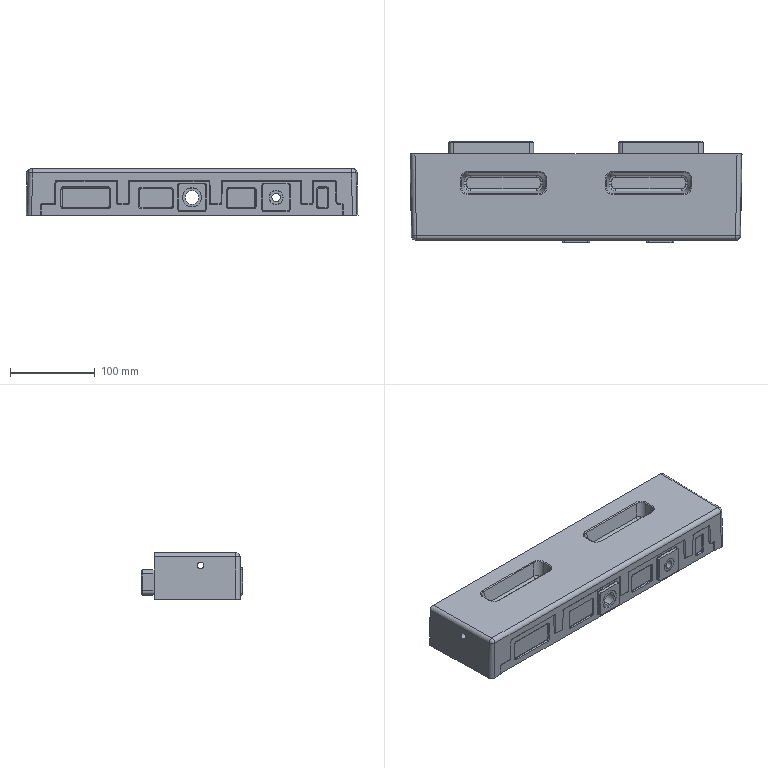Part | SolidWorks | features BaseBody 1 | 1 solid | 339 faces | box 392.349 x 119.708 x 55 mm | volume 2097118 mm3 | cylinder 130 | plane 77 | torus 64 | cone 30 | spline 28 | sphere 10 | commonest cylinder face diameters 2.011 x34 1.005 x27 10 x15 8 x14 16 x12 6 x10